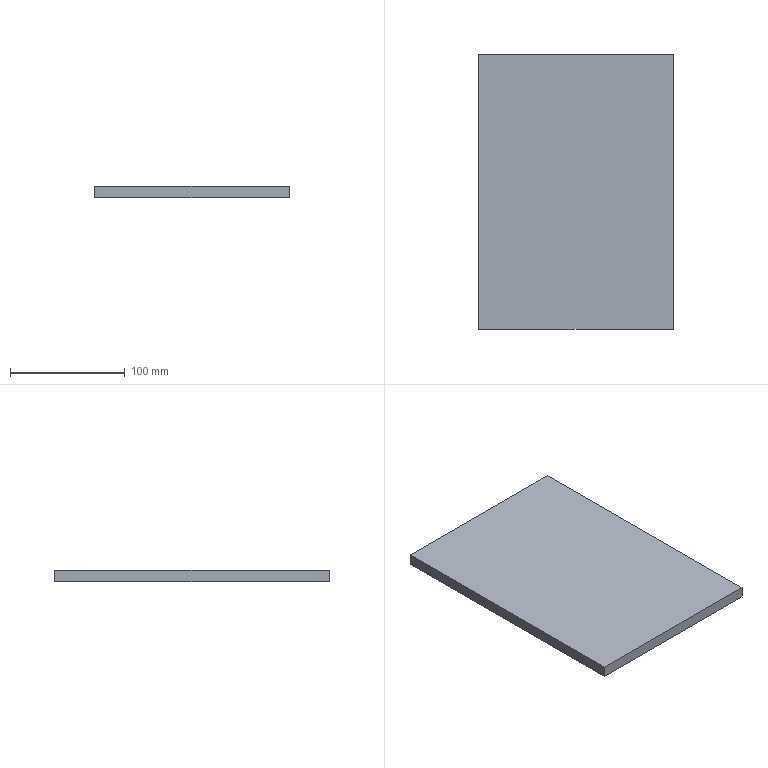Part | SolidWorks | features Extrusion 1 | 1 solid | 6 faces | box 170 x 240 x 10 mm | volume 408000 mm3 | plane 6
STEP:
#1=CARTESIAN_POINT('',(-85.,120.,0.));
#2=VERTEX_POINT('',#1);
#3=CARTESIAN_POINT('',(-85.,-120.,0.));
#4=VERTEX_POINT('',#3);
#5=CARTESIAN_POINT('',(-85.,120.,0.));
#6=DIRECTION('',(0.,-1.,0.));
#7=VECTOR('',#6,1000.);
#8=LINE('',#5,#7);
#9=EDGE_CURVE('',#2,#4,#8,.T.);
#10=ORIENTED_EDGE('',*,*,#9,.T.);
#11=CARTESIAN_POINT('',(-85.,-120.,10.));
#12=VERTEX_POINT('',#11);
#13=CARTESIAN_POINT('',(-85.,-120.,10.));
#14=DIRECTION('',(0.,0.,-1.));
#15=VECTOR('',#14,1000.);
#16=LINE('',#13,#15);
#17=EDGE_CURVE('',#12,#4,#16,.T.);
#18=ORIENTED_EDGE('',*,*,#17,.F.);
#19=CARTESIAN_POINT('',(-85.,120.,10.));
#20=VERTEX_POINT('',#19);
#21=CARTESIAN_POINT('',(-85.,120.,10.));
#22=DIRECTION('',(0.,-1.,0.));
#23=VECTOR('',#22,1000.);
#24=LINE('',#21,#23);
#25=EDGE_CURVE('',#20,#12,#24,.T.);
#26=ORIENTED_EDGE('',*,*,#25,.F.);
#27=CARTESIAN_POINT('',(-85.,120.,10.));
#28=DIRECTION('',(0.,0.,-1.));
#29=VECTOR('',#28,1000.);
#30=LINE('',#27,#29);
#31=EDGE_CURVE('',#20,#2,#30,.T.);
#32=ORIENTED_EDGE('',*,*,#31,.T.);
#33=EDGE_LOOP('',(#10,#18,#26,#32));
#34=FACE_OUTER_BOUND('',#33,.T.);
#35=CARTESIAN_POINT('',(-85.,120.,10.));
#36=DIRECTION('',(1.,0.,0.));
#37=DIRECTION('',(0.,1.,0.));
#38=AXIS2_PLACEMENT_3D('',#35,#36,#37);
#39=PLANE('',#38);
#40=ADVANCED_FACE('',(#34),#39,.F.);
#41=CARTESIAN_POINT('',(85.,-120.,0.));
#42=VERTEX_POINT('',#41);
#43=CARTESIAN_POINT('',(85.,-120.,0.));
#44=DIRECTION('',(1.,0.,0.));
#45=VECTOR('',#44,1000.);
#46=LINE('',#43,#45);
#47=EDGE_CURVE('',#4,#42,#46,.T.);
#48=ORIENTED_EDGE('',*,*,#47,.T.);
#49=CARTESIAN_POINT('',(85.,-120.,10.));
#50=VERTEX_POINT('',#49);
#51=CARTESIAN_POINT('',(85.,-120.,10.));
#52=DIRECTION('',(0.,0.,-1.));
#53=VECTOR('',#52,1000.);
#54=LINE('',#51,#53);
#55=EDGE_CURVE('',#50,#42,#54,.T.);
#56=ORIENTED_EDGE('',*,*,#55,.F.);
#57=CARTESIAN_POINT('',(85.,-120.,10.));
#58=DIRECTION('',(1.,0.,0.));
#59=VECTOR('',#58,1000.);
#60=LINE('',#57,#59);
#61=EDGE_CURVE('',#12,#50,#60,.T.);
#62=ORIENTED_EDGE('',*,*,#61,.F.);
#63=ORIENTED_EDGE('',*,*,#17,.T.);
#64=EDGE_LOOP('',(#48,#56,#62,#63));
#65=FACE_OUTER_BOUND('',#64,.T.);
#66=CARTESIAN_POINT('',(85.,-120.,10.));
#67=DIRECTION('',(0.,1.,0.));
#68=DIRECTION('',(-1.,0.,0.));
#69=AXIS2_PLACEMENT_3D('',#66,#67,#68);
#70=PLANE('',#69);
#71=ADVANCED_FACE('',(#65),#70,.F.);
#72=CARTESIAN_POINT('',(85.,120.,0.));
#73=VERTEX_POINT('',#72);
#74=CARTESIAN_POINT('',(85.,120.,0.));
#75=DIRECTION('',(0.,1.,0.));
#76=VECTOR('',#75,1000.);
#77=LINE('',#74,#76);
#78=EDGE_CURVE('',#42,#73,#77,.T.);
#79=ORIENTED_EDGE('',*,*,#78,.T.);
#80=CARTESIAN_POINT('',(85.,120.,10.));
#81=VERTEX_POINT('',#80);
#82=CARTESIAN_POINT('',(85.,120.,10.));
#83=DIRECTION('',(0.,0.,-1.));
#84=VECTOR('',#83,1000.);
#85=LINE('',#82,#84);
#86=EDGE_CURVE('',#81,#73,#85,.T.);
#87=ORIENTED_EDGE('',*,*,#86,.F.);
#88=CARTESIAN_POINT('',(85.,120.,10.));
#89=DIRECTION('',(0.,1.,0.));
#90=VECTOR('',#89,1000.);
#91=LINE('',#88,#90);
#92=EDGE_CURVE('',#50,#81,#91,.T.);
#93=ORIENTED_EDGE('',*,*,#92,.F.);
#94=ORIENTED_EDGE('',*,*,#55,.T.);
#95=EDGE_LOOP('',(#79,#87,#93,#94));
#96=FACE_OUTER_BOUND('',#95,.T.);
#97=CARTESIAN_POINT('',(85.,120.,10.));
#98=DIRECTION('',(-1.,0.,0.));
#99=DIRECTION('',(0.,-1.,0.));
#100=AXIS2_PLACEMENT_3D('',#97,#98,#99);
#101=PLANE('',#100);
#102=ADVANCED_FACE('',(#96),#101,.F.);
#103=CARTESIAN_POINT('',(85.,120.,0.));
#104=DIRECTION('',(-1.,0.,0.));
#105=VECTOR('',#104,1000.);
#106=LINE('',#103,#105);
#107=EDGE_CURVE('',#73,#2,#106,.T.);
#108=ORIENTED_EDGE('',*,*,#107,.T.);
#109=ORIENTED_EDGE('',*,*,#31,.F.);
#110=CARTESIAN_POINT('',(85.,120.,10.));
#111=DIRECTION('',(-1.,0.,0.));
#112=VECTOR('',#111,1000.);
#113=LINE('',#110,#112);
#114=EDGE_CURVE('',#81,#20,#113,.T.);
#115=ORIENTED_EDGE('',*,*,#114,.F.);
#116=ORIENTED_EDGE('',*,*,#86,.T.);
#117=EDGE_LOOP('',(#108,#109,#115,#116));
#118=FACE_OUTER_BOUND('',#117,.T.);
#119=CARTESIAN_POINT('',(85.,120.,10.));
#120=DIRECTION('',(0.,-1.,0.));
#121=DIRECTION('',(1.,0.,0.));
#122=AXIS2_PLACEMENT_3D('',#119,#120,#121);
#123=PLANE('',#122);
#124=ADVANCED_FACE('',(#118),#123,.F.);
#125=ORIENTED_EDGE('',*,*,#25,.T.);
#126=ORIENTED_EDGE('',*,*,#61,.T.);
#127=ORIENTED_EDGE('',*,*,#92,.T.);
#128=ORIENTED_EDGE('',*,*,#114,.T.);
#129=EDGE_LOOP('',(#125,#126,#127,#128));
#130=FACE_OUTER_BOUND('',#129,.T.);
#131=CARTESIAN_POINT('',(0.,0.,10.));
#132=DIRECTION('',(0.,0.,-1.));
#133=DIRECTION('',(-1.,0.,0.));
#134=AXIS2_PLACEMENT_3D('',#131,#132,#133);
#135=PLANE('',#134);
#136=ADVANCED_FACE('',(#130),#135,.F.);
#137=ORIENTED_EDGE('',*,*,#9,.F.);
#138=ORIENTED_EDGE('',*,*,#107,.F.);
#139=ORIENTED_EDGE('',*,*,#78,.F.);
#140=ORIENTED_EDGE('',*,*,#47,.F.);
#141=EDGE_LOOP('',(#137,#138,#139,#140));
#142=FACE_OUTER_BOUND('',#141,.T.);
#143=CARTESIAN_POINT('',(0.,0.,0.));
#144=DIRECTION('',(0.,0.,-1.));
#145=DIRECTION('',(-1.,0.,0.));
#146=AXIS2_PLACEMENT_3D('',#143,#144,#145);
#147=PLANE('',#146);
#148=ADVANCED_FACE('',(#142),#147,.T.);
#149=CLOSED_SHELL('',(#40,#71,#102,#124,#136,#148));
#150=MANIFOLD_SOLID_BREP('',#149);
#151=CARTESIAN_POINT('',(0.,0.,0.));
#152=DIRECTION('',(0.,0.,1.));
#153=DIRECTION('',(1.,0.,0.));
#154=AXIS2_PLACEMENT_3D('',#151,#152,#153);
#155=(LENGTH_UNIT()NAMED_UNIT(*)SI_UNIT(.MILLI.,.METRE.));
#156=UNCERTAINTY_MEASURE_WITH_UNIT(LENGTH_MEASURE(0.00001),#155,'','');
#157=(NAMED_UNIT(*)PLANE_ANGLE_UNIT()SI_UNIT($,.RADIAN.));
#158=(NAMED_UNIT(*)SI_UNIT($,.STERADIAN.)SOLID_ANGLE_UNIT());
#159=(GEOMETRIC_REPRESENTATION_CONTEXT(3)GLOBAL_UNCERTAINTY_ASSIGNED_CONTEXT((#156))GLOBAL_UNIT_ASSIGNED_CONTEXT((#155,#157,#158))REPRESENTATION_CONTEXT('',''));
#160=ADVANCED_BREP_SHAPE_REPRESENTATION('',(#150,#154),#159);